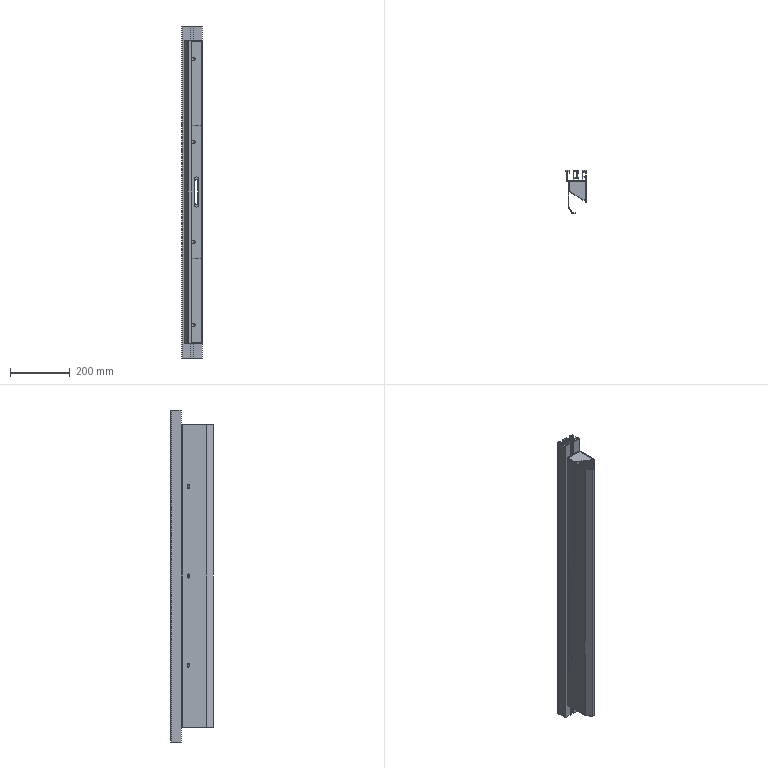Part | 7 solids | 251 faces | box 70 x 143.651 x 1115 mm | volume 1401720 mm3 | plane 168 | cylinder 83 | commonest cylinder face diameters 10 x31 7 x12 6 x11 2 x8 3 x7 5 x4